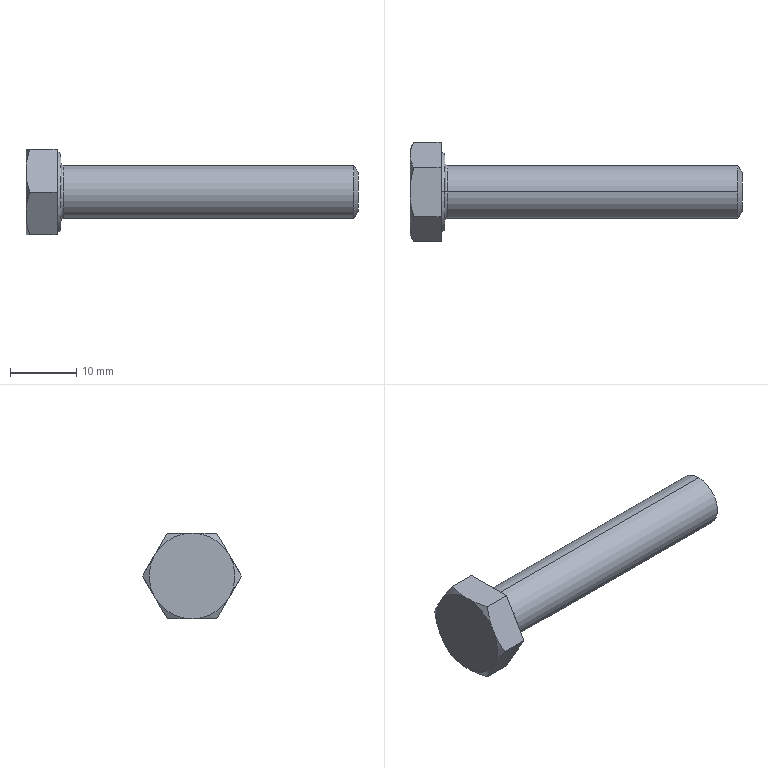Part | SolidWorks | features BaseBody 1 | 1 solid | 24 faces | box 50.3 x 15.011 x 13 mm | volume 3008 mm3 | cone 10 | plane 10 | spline 2 | cylinder 2 | commonest cylinder face diameters 8 x2
STEP:
#1=CARTESIAN_POINT('',(5.3,0.,4.4));
#2=VERTEX_POINT('',#1);
#3=CARTESIAN_POINT('',(5.3,0.,-4.4));
#4=VERTEX_POINT('',#3);
#5=CARTESIAN_POINT('',(5.3,0.,4.4));
#6=CARTESIAN_POINT('',(5.3,0.2797,4.4));
#7=CARTESIAN_POINT('',(5.3,0.6919,4.361));
#8=CARTESIAN_POINT('',(5.3,1.16,4.249));
#9=CARTESIAN_POINT('',(5.3,1.391,4.176));
#10=CARTESIAN_POINT('',(5.3,1.489,4.141));
#11=CARTESIAN_POINT('',(5.3,1.554,4.116));
#12=CARTESIAN_POINT('',(5.3,1.585,4.105));
#13=CARTESIAN_POINT('',(5.3,1.758,4.036));
#14=CARTESIAN_POINT('',(5.3,1.96,3.944));
#15=CARTESIAN_POINT('',(5.3,2.154,3.837));
#16=CARTESIAN_POINT('',(5.3,2.282,3.763));
#17=CARTESIAN_POINT('',(5.3,2.344,3.724));
#18=CARTESIAN_POINT('',(5.3,2.662,3.517));
#19=CARTESIAN_POINT('',(5.3,2.897,3.326));
#20=CARTESIAN_POINT('',(5.3,3.219,3.004));
#21=CARTESIAN_POINT('',(5.3,3.37,2.836));
#22=CARTESIAN_POINT('',(5.3,3.509,2.656));
#23=CARTESIAN_POINT('',(5.3,3.598,2.534));
#24=CARTESIAN_POINT('',(5.3,3.642,2.47));
#25=CARTESIAN_POINT('',(5.3,3.764,2.283));
#26=CARTESIAN_POINT('',(5.3,3.876,2.092));
#27=CARTESIAN_POINT('',(5.3,3.989,1.859));
#28=CARTESIAN_POINT('',(5.3,4.042,1.74));
#29=CARTESIAN_POINT('',(5.3,4.063,1.689));
#30=CARTESIAN_POINT('',(5.3,4.077,1.654));
#31=CARTESIAN_POINT('',(5.3,4.085,1.636));
#32=CARTESIAN_POINT('',(5.3,4.297,1.1));
#33=CARTESIAN_POINT('',(5.3,4.4,0.5592));
#34=CARTESIAN_POINT('',(5.3,4.4,-0.2796));
#35=CARTESIAN_POINT('',(5.3,4.361,-0.6917));
#36=CARTESIAN_POINT('',(5.3,4.249,-1.16));
#37=CARTESIAN_POINT('',(5.3,4.176,-1.391));
#38=CARTESIAN_POINT('',(5.3,4.141,-1.489));
#39=CARTESIAN_POINT('',(5.3,4.116,-1.554));
#40=CARTESIAN_POINT('',(5.3,4.105,-1.585));
#41=CARTESIAN_POINT('',(5.3,4.036,-1.758));
#42=CARTESIAN_POINT('',(5.3,3.944,-1.96));
#43=CARTESIAN_POINT('',(5.3,3.837,-2.154));
#44=CARTESIAN_POINT('',(5.3,3.763,-2.282));
#45=CARTESIAN_POINT('',(5.3,3.724,-2.344));
#46=CARTESIAN_POINT('',(5.3,3.517,-2.662));
#47=CARTESIAN_POINT('',(5.3,3.326,-2.897));
#48=CARTESIAN_POINT('',(5.3,3.004,-3.219));
#49=CARTESIAN_POINT('',(5.3,2.836,-3.37));
#50=CARTESIAN_POINT('',(5.3,2.656,-3.509));
#51=CARTESIAN_POINT('',(5.3,2.534,-3.598));
#52=CARTESIAN_POINT('',(5.3,2.47,-3.642));
#53=CARTESIAN_POINT('',(5.3,2.283,-3.764));
#54=CARTESIAN_POINT('',(5.3,2.092,-3.876));
#55=CARTESIAN_POINT('',(5.3,1.859,-3.989));
#56=CARTESIAN_POINT('',(5.3,1.74,-4.042));
#57=CARTESIAN_POINT('',(5.3,1.689,-4.063));
#58=CARTESIAN_POINT('',(5.3,1.654,-4.077));
#59=CARTESIAN_POINT('',(5.3,1.636,-4.085));
#60=CARTESIAN_POINT('',(5.3,1.1,-4.297));
#61=CARTESIAN_POINT('',(5.3,0.5597,-4.4));
#62=CARTESIAN_POINT('',(5.3,0.,-4.4));
#63=B_SPLINE_CURVE_WITH_KNOTS('',3,(#5,#6,#7,#8,#9,#10,#11,#12,#13,#14,#15,#16,#17,#18,#19,#20,#21,#22,#23,#24,#25,#26,#27,#28,#29,#30,#31,#32,#33,#34,#35,#36,#37,#38,#39,#40,#41,#42,#43,#44,#45,#46,#47,#48,#49,#50,#51,#52,#53,#54,#55,#56,#57,#58,#59,#60,#61,#62),.UNSPECIFIED.,.F.,.F.,(4,1,1,1,2,2,1,2,2,2,1,2,2,1,1,1,2,2,2,1,1,1,2,2,1,2,2,2,1,2,2,1,1,1,2,2,4),(0.,0.0625,0.09375,0.1094,0.1172,0.125,0.1562,0.1719,0.1875,0.25,0.2812,0.2969,0.3125,0.3437,0.3594,0.3672,0.3711,0.375,0.5,0.5625,0.5937,0.6094,0.6172,0.625,0.6562,0.6719,0.6875,0.75,0.7812,0.7969,0.8125,0.8437,0.8594,0.8672,0.8711,0.875,1.),.UNSPECIFIED.);
#64=EDGE_CURVE('',#2,#4,#63,.T.);
#65=ORIENTED_EDGE('',*,*,#64,.F.);
#66=CARTESIAN_POINT('',(5.7,0.,4.));
#67=VERTEX_POINT('',#66);
#68=CARTESIAN_POINT('',(5.7,0.,4.4));
#69=DIRECTION('',(0.,-1.,0.));
#70=DIRECTION('',(0.,0.,1.));
#71=AXIS2_PLACEMENT_3D('',#68,#69,#70);
#72=CIRCLE('',#71,0.4);
#73=EDGE_CURVE('',#2,#67,#72,.T.);
#74=ORIENTED_EDGE('',*,*,#73,.T.);
#75=CARTESIAN_POINT('',(5.7,0.,-4.));
#76=VERTEX_POINT('',#75);
#77=CARTESIAN_POINT('',(5.7,0.,0.));
#78=DIRECTION('',(1.,0.,0.));
#79=DIRECTION('',(0.,0.,1.));
#80=AXIS2_PLACEMENT_3D('',#77,#78,#79);
#81=CIRCLE('',#80,4.);
#82=EDGE_CURVE('',#76,#67,#81,.T.);
#83=ORIENTED_EDGE('',*,*,#82,.F.);
#84=CARTESIAN_POINT('',(5.7,0.,-4.4));
#85=DIRECTION('',(0.,1.,0.));
#86=DIRECTION('',(0.,0.,-1.));
#87=AXIS2_PLACEMENT_3D('',#84,#85,#86);
#88=CIRCLE('',#87,0.4);
#89=EDGE_CURVE('',#4,#76,#88,.T.);
#90=ORIENTED_EDGE('',*,*,#89,.F.);
#91=EDGE_LOOP('',(#65,#74,#83,#90));
#92=FACE_OUTER_BOUND('',#91,.T.);
#93=CARTESIAN_POINT('',(5.3,0.,-4.4));
#94=CARTESIAN_POINT('',(5.3,8.8,-4.4));
#95=CARTESIAN_POINT('',(5.3,8.8,4.4));
#96=CARTESIAN_POINT('',(5.3,0.,4.4));
#97=CARTESIAN_POINT('',(5.3,0.,-4.166));
#98=CARTESIAN_POINT('',(5.3,8.331,-4.166));
#99=CARTESIAN_POINT('',(5.3,8.331,4.166));
#100=CARTESIAN_POINT('',(5.3,0.,4.166));
#101=CARTESIAN_POINT('',(5.466,0.,-4.));
#102=CARTESIAN_POINT('',(5.466,8.,-4.));
#103=CARTESIAN_POINT('',(5.466,8.,4.));
#104=CARTESIAN_POINT('',(5.466,0.,4.));
#105=CARTESIAN_POINT('',(5.7,0.,-4.));
#106=CARTESIAN_POINT('',(5.7,8.,-4.));
#107=CARTESIAN_POINT('',(5.7,8.,4.));
#108=CARTESIAN_POINT('',(5.7,0.,4.));
#109=(BOUNDED_SURFACE()B_SPLINE_SURFACE(3,3,((#93,#94,#95,#96),(#97,#98,#99,#100),(#101,#102,#103,#104),(#105,#106,#107,#108)),.UNSPECIFIED.,.F.,.F.,.F.)B_SPLINE_SURFACE_WITH_KNOTS((4,4),(4,4),(0.,1.),(0.,1.),.UNSPECIFIED.)GEOMETRIC_REPRESENTATION_ITEM()RATIONAL_B_SPLINE_SURFACE(((1.,0.3333,0.3333,1.),(0.8047,0.2682,0.2682,0.8047),(0.8047,0.2682,0.2682,0.8047),(1.,0.3333,0.3333,1.)))REPRESENTATION_ITEM('')SURFACE());
#110=ADVANCED_FACE('',(#92),#109,.F.);
#111=CARTESIAN_POINT('',(49.675,0.,4.));
#112=VERTEX_POINT('',#111);
#113=CARTESIAN_POINT('',(49.675,0.,-4.));
#114=VERTEX_POINT('',#113);
#115=CARTESIAN_POINT('',(49.675,0.,0.));
#116=DIRECTION('',(-1.,0.,0.));
#117=DIRECTION('',(0.,0.,1.));
#118=AXIS2_PLACEMENT_3D('',#115,#116,#117);
#119=CIRCLE('',#118,4.);
#120=EDGE_CURVE('',#112,#114,#119,.T.);
#121=ORIENTED_EDGE('',*,*,#120,.T.);
#122=CARTESIAN_POINT('',(0.,0.,-4.));
#123=DIRECTION('',(-1.,0.,0.));
#124=VECTOR('',#123,1000.);
#125=LINE('',#122,#124);
#126=EDGE_CURVE('',#114,#76,#125,.T.);
#127=ORIENTED_EDGE('',*,*,#126,.T.);
#128=ORIENTED_EDGE('',*,*,#82,.T.);
#129=CARTESIAN_POINT('',(0.,0.,4.));
#130=DIRECTION('',(-1.,0.,0.));
#131=VECTOR('',#130,1000.);
#132=LINE('',#129,#131);
#133=EDGE_CURVE('',#112,#67,#132,.T.);
#134=ORIENTED_EDGE('',*,*,#133,.F.);
#135=EDGE_LOOP('',(#121,#127,#128,#134));
#136=FACE_OUTER_BOUND('',#135,.T.);
#137=CARTESIAN_POINT('',(0.,0.,0.));
#138=DIRECTION('',(-1.,0.,0.));
#139=DIRECTION('',(0.,0.,1.));
#140=AXIS2_PLACEMENT_3D('',#137,#138,#139);
#141=CYLINDRICAL_SURFACE('',#140,4.);
#142=ADVANCED_FACE('',(#136),#141,.T.);
#143=CARTESIAN_POINT('',(50.3,0.,2.917));
#144=VERTEX_POINT('',#143);
#145=CARTESIAN_POINT('',(50.3,0.,-2.917));
#146=VERTEX_POINT('',#145);
#147=CARTESIAN_POINT('',(50.3,0.,0.));
#148=DIRECTION('',(-1.,0.,0.));
#149=DIRECTION('',(0.,0.,1.));
#150=AXIS2_PLACEMENT_3D('',#147,#148,#149);
#151=CIRCLE('',#150,2.917);
#152=EDGE_CURVE('',#144,#146,#151,.T.);
#153=ORIENTED_EDGE('',*,*,#152,.T.);
#154=CARTESIAN_POINT('',(49.675,0.,-4.));
#155=DIRECTION('',(-0.5,0.,-0.866));
#156=VECTOR('',#155,1000.);
#157=LINE('',#154,#156);
#158=EDGE_CURVE('',#146,#114,#157,.T.);
#159=ORIENTED_EDGE('',*,*,#158,.T.);
#160=ORIENTED_EDGE('',*,*,#120,.F.);
#161=CARTESIAN_POINT('',(49.675,0.,4.));
#162=DIRECTION('',(-0.5,0.,0.866));
#163=VECTOR('',#162,1000.);
#164=LINE('',#161,#163);
#165=EDGE_CURVE('',#144,#112,#164,.T.);
#166=ORIENTED_EDGE('',*,*,#165,.F.);
#167=EDGE_LOOP('',(#153,#159,#160,#166));
#168=FACE_OUTER_BOUND('',#167,.T.);
#169=CARTESIAN_POINT('',(49.675,0.,0.));
#170=DIRECTION('',(-1.,0.,0.));
#171=DIRECTION('',(0.,0.,1.));
#172=AXIS2_PLACEMENT_3D('',#169,#170,#171);
#173=CONICAL_SURFACE('',#172,4.,1.047);
#174=ADVANCED_FACE('',(#168),#173,.T.);
#175=CARTESIAN_POINT('',(5.3,0.,-5.815));
#176=VERTEX_POINT('',#175);
#177=CARTESIAN_POINT('',(5.3,0.,5.815));
#178=VERTEX_POINT('',#177);
#179=CARTESIAN_POINT('',(5.3,0.,0.));
#180=DIRECTION('',(1.,0.,0.));
#181=DIRECTION('',(0.,0.,1.));
#182=AXIS2_PLACEMENT_3D('',#179,#180,#181);
#183=CIRCLE('',#182,5.815);
#184=EDGE_CURVE('',#176,#178,#183,.T.);
#185=ORIENTED_EDGE('',*,*,#184,.F.);
#186=CARTESIAN_POINT('',(4.7,0.,-6.161));
#187=VERTEX_POINT('',#186);
#188=CARTESIAN_POINT('',(4.7,0.,-6.161));
#189=DIRECTION('',(-0.866,0.,-0.5));
#190=VECTOR('',#189,1000.);
#191=LINE('',#188,#190);
#192=EDGE_CURVE('',#176,#187,#191,.T.);
#193=ORIENTED_EDGE('',*,*,#192,.T.);
#194=CARTESIAN_POINT('',(4.7,0.,6.161));
#195=VERTEX_POINT('',#194);
#196=CARTESIAN_POINT('',(4.7,0.,0.));
#197=DIRECTION('',(1.,0.,0.));
#198=DIRECTION('',(0.,0.,1.));
#199=AXIS2_PLACEMENT_3D('',#196,#197,#198);
#200=CIRCLE('',#199,6.161);
#201=EDGE_CURVE('',#187,#195,#200,.T.);
#202=ORIENTED_EDGE('',*,*,#201,.T.);
#203=CARTESIAN_POINT('',(4.7,0.,6.161));
#204=DIRECTION('',(-0.866,0.,0.5));
#205=VECTOR('',#204,1000.);
#206=LINE('',#203,#205);
#207=EDGE_CURVE('',#178,#195,#206,.T.);
#208=ORIENTED_EDGE('',*,*,#207,.F.);
#209=EDGE_LOOP('',(#185,#193,#202,#208));
#210=FACE_OUTER_BOUND('',#209,.T.);
#211=CARTESIAN_POINT('',(4.7,0.,0.));
#212=DIRECTION('',(-1.,0.,0.));
#213=DIRECTION('',(0.,0.,1.));
#214=AXIS2_PLACEMENT_3D('',#211,#212,#213);
#215=CONICAL_SURFACE('',#214,6.161,0.5236);
#216=ADVANCED_FACE('',(#210),#215,.T.);
#217=ORIENTED_EDGE('',*,*,#126,.F.);
#218=CARTESIAN_POINT('',(49.675,0.,0.));
#219=DIRECTION('',(-1.,0.,0.));
#220=DIRECTION('',(0.,0.,1.));
#221=AXIS2_PLACEMENT_3D('',#218,#219,#220);
#222=CIRCLE('',#221,4.);
#223=EDGE_CURVE('',#114,#112,#222,.T.);
#224=ORIENTED_EDGE('',*,*,#223,.T.);
#225=ORIENTED_EDGE('',*,*,#133,.T.);
#226=CARTESIAN_POINT('',(5.7,0.,0.));
#227=DIRECTION('',(1.,0.,0.));
#228=DIRECTION('',(0.,0.,1.));
#229=AXIS2_PLACEMENT_3D('',#226,#227,#228);
#230=CIRCLE('',#229,4.);
#231=EDGE_CURVE('',#67,#76,#230,.T.);
#232=ORIENTED_EDGE('',*,*,#231,.T.);
#233=EDGE_LOOP('',(#217,#224,#225,#232));
#234=FACE_OUTER_BOUND('',#233,.T.);
#235=CARTESIAN_POINT('',(0.,0.,0.));
#236=DIRECTION('',(-1.,0.,0.));
#237=DIRECTION('',(0.,0.,1.));
#238=AXIS2_PLACEMENT_3D('',#235,#236,#237);
#239=CYLINDRICAL_SURFACE('',#238,4.);
#240=ADVANCED_FACE('',(#234),#239,.T.);
#241=ORIENTED_EDGE('',*,*,#73,.F.);
#242=CARTESIAN_POINT('',(5.3,0.,-4.4));
#243=CARTESIAN_POINT('',(5.3,-0.2797,-4.4));
#244=CARTESIAN_POINT('',(5.3,-0.6919,-4.361));
#245=CARTESIAN_POINT('',(5.3,-1.16,-4.249));
#246=CARTESIAN_POINT('',(5.3,-1.391,-4.176));
#247=CARTESIAN_POINT('',(5.3,-1.489,-4.141));
#248=CARTESIAN_POINT('',(5.3,-1.554,-4.116));
#249=CARTESIAN_POINT('',(5.3,-1.585,-4.105));
#250=CARTESIAN_POINT('',(5.3,-1.758,-4.036));
#251=CARTESIAN_POINT('',(5.3,-1.96,-3.944));
#252=CARTESIAN_POINT('',(5.3,-2.154,-3.837));
#253=CARTESIAN_POINT('',(5.3,-2.282,-3.763));
#254=CARTESIAN_POINT('',(5.3,-2.344,-3.724));
#255=CARTESIAN_POINT('',(5.3,-2.662,-3.517));
#256=CARTESIAN_POINT('',(5.3,-2.897,-3.326));
#257=CARTESIAN_POINT('',(5.3,-3.219,-3.004));
#258=CARTESIAN_POINT('',(5.3,-3.37,-2.836));
#259=CARTESIAN_POINT('',(5.3,-3.509,-2.656));
#260=CARTESIAN_POINT('',(5.3,-3.598,-2.534));
#261=CARTESIAN_POINT('',(5.3,-3.642,-2.47));
#262=CARTESIAN_POINT('',(5.3,-3.764,-2.283));
#263=CARTESIAN_POINT('',(5.3,-3.876,-2.092));
#264=CARTESIAN_POINT('',(5.3,-3.989,-1.859));
#265=CARTESIAN_POINT('',(5.3,-4.042,-1.74));
#266=CARTESIAN_POINT('',(5.3,-4.063,-1.689));
#267=CARTESIAN_POINT('',(5.3,-4.077,-1.654));
#268=CARTESIAN_POINT('',(5.3,-4.085,-1.636));
#269=CARTESIAN_POINT('',(5.3,-4.297,-1.1));
#270=CARTESIAN_POINT('',(5.3,-4.4,-0.5592));
#271=CARTESIAN_POINT('',(5.3,-4.4,0.2796));
#272=CARTESIAN_POINT('',(5.3,-4.361,0.6917));
#273=CARTESIAN_POINT('',(5.3,-4.249,1.16));
#274=CARTESIAN_POINT('',(5.3,-4.176,1.391));
#275=CARTESIAN_POINT('',(5.3,-4.141,1.489));
#276=CARTESIAN_POINT('',(5.3,-4.116,1.554));
#277=CARTESIAN_POINT('',(5.3,-4.105,1.585));
#278=CARTESIAN_POINT('',(5.3,-4.036,1.758));
#279=CARTESIAN_POINT('',(5.3,-3.944,1.96));
#280=CARTESIAN_POINT('',(5.3,-3.837,2.154));
#281=CARTESIAN_POINT('',(5.3,-3.763,2.282));
#282=CARTESIAN_POINT('',(5.3,-3.724,2.344));
#283=CARTESIAN_POINT('',(5.3,-3.517,2.662));
#284=CARTESIAN_POINT('',(5.3,-3.326,2.897));
#285=CARTESIAN_POINT('',(5.3,-3.004,3.219));
#286=CARTESIAN_POINT('',(5.3,-2.836,3.37));
#287=CARTESIAN_POINT('',(5.3,-2.656,3.509));
#288=CARTESIAN_POINT('',(5.3,-2.534,3.598));
#289=CARTESIAN_POINT('',(5.3,-2.47,3.642));
#290=CARTESIAN_POINT('',(5.3,-2.283,3.764));
#291=CARTESIAN_POINT('',(5.3,-2.092,3.876));
#292=CARTESIAN_POINT('',(5.3,-1.859,3.989));
#293=CARTESIAN_POINT('',(5.3,-1.74,4.042));
#294=CARTESIAN_POINT('',(5.3,-1.689,4.063));
#295=CARTESIAN_POINT('',(5.3,-1.654,4.077));
#296=CARTESIAN_POINT('',(5.3,-1.636,4.085));
#297=CARTESIAN_POINT('',(5.3,-1.1,4.297));
#298=CARTESIAN_POINT('',(5.3,-0.5597,4.4));
#299=CARTESIAN_POINT('',(5.3,0.,4.4));
#300=B_SPLINE_CURVE_WITH_KNOTS('',3,(#242,#243,#244,#245,#246,#247,#248,#249,#250,#251,#252,#253,#254,#255,#256,#257,#258,#259,#260,#261,#262,#263,#264,#265,#266,#267,#268,#269,#270,#271,#272,#273,#274,#275,#276,#277,#278,#279,#280,#281,#282,#283,#284,#285,#286,#287,#288,#289,#290,#291,#292,#293,#294,#295,#296,#297,#298,#299),.UNSPECIFIED.,.F.,.F.,(4,1,1,1,2,2,1,2,2,2,1,2,2,1,1,1,2,2,2,1,1,1,2,2,1,2,2,2,1,2,2,1,1,1,2,2,4),(0.,0.0625,0.09375,0.1094,0.1172,0.125,0.1562,0.1719,0.1875,0.25,0.2812,0.2969,0.3125,0.3437,0.3594,0.3672,0.3711,0.375,0.5,0.5625,0.5937,0.6094,0.6172,0.625,0.6562,0.6719,0.6875,0.75,0.7812,0.7969,0.8125,0.8437,0.8594,0.8672,0.8711,0.875,1.),.UNSPECIFIED.);
#301=EDGE_CURVE('',#4,#2,#300,.T.);
#302=ORIENTED_EDGE('',*,*,#301,.F.);
#303=ORIENTED_EDGE('',*,*,#89,.T.);
#304=ORIENTED_EDGE('',*,*,#231,.F.);
#305=EDGE_LOOP('',(#241,#302,#303,#304));
#306=FACE_OUTER_BOUND('',#305,.T.);
#307=CARTESIAN_POINT('',(5.3,0.,4.4));
#308=CARTESIAN_POINT('',(5.3,-8.8,4.4));
#309=CARTESIAN_POINT('',(5.3,-8.8,-4.4));
#310=CARTESIAN_POINT('',(5.3,0.,-4.4));
#311=CARTESIAN_POINT('',(5.3,0.,4.166));
#312=CARTESIAN_POINT('',(5.3,-8.331,4.166));
#313=CARTESIAN_POINT('',(5.3,-8.331,-4.166));
#314=CARTESIAN_POINT('',(5.3,0.,-4.166));
#315=CARTESIAN_POINT('',(5.466,0.,4.));
#316=CARTESIAN_POINT('',(5.466,-8.,4.));
#317=CARTESIAN_POINT('',(5.466,-8.,-4.));
#318=CARTESIAN_POINT('',(5.466,0.,-4.));
#319=CARTESIAN_POINT('',(5.7,0.,4.));
#320=CARTESIAN_POINT('',(5.7,-8.,4.));
#321=CARTESIAN_POINT('',(5.7,-8.,-4.));
#322=CARTESIAN_POINT('',(5.7,0.,-4.));
#323=(BOUNDED_SURFACE()B_SPLINE_SURFACE(3,3,((#307,#308,#309,#310),(#311,#312,#313,#314),(#315,#316,#317,#318),(#319,#320,#321,#322)),.UNSPECIFIED.,.F.,.F.,.T.)B_SPLINE_SURFACE_WITH_KNOTS((4,4),(4,4),(0.,1.),(0.,1.),.UNSPECIFIED.)GEOMETRIC_REPRESENTATION_ITEM()RATIONAL_B_SPLINE_SURFACE(((1.,0.3333,0.3333,1.),(0.8047,0.2682,0.2682,0.8047),(0.8047,0.2682,0.2682,0.8047),(1.,0.3333,0.3333,1.)))REPRESENTATION_ITEM('')SURFACE());
#324=ADVANCED_FACE('',(#306),#323,.F.);
#325=ORIENTED_EDGE('',*,*,#158,.F.);
#326=CARTESIAN_POINT('',(50.3,0.,0.));
#327=DIRECTION('',(-1.,0.,0.));
#328=DIRECTION('',(0.,0.,1.));
#329=AXIS2_PLACEMENT_3D('',#326,#327,#328);
#330=CIRCLE('',#329,2.917);
#331=EDGE_CURVE('',#146,#144,#330,.T.);
#332=ORIENTED_EDGE('',*,*,#331,.T.);
#333=ORIENTED_EDGE('',*,*,#165,.T.);
#334=ORIENTED_EDGE('',*,*,#223,.F.);
#335=EDGE_LOOP('',(#325,#332,#333,#334));
#336=FACE_OUTER_BOUND('',#335,.T.);
#337=CARTESIAN_POINT('',(49.675,0.,0.));
#338=DIRECTION('',(-1.,0.,0.));
#339=DIRECTION('',(0.,0.,1.));
#340=AXIS2_PLACEMENT_3D('',#337,#338,#339);
#341=CONICAL_SURFACE('',#340,4.,1.047);
#342=ADVANCED_FACE('',(#336),#341,.T.);
#343=CARTESIAN_POINT('',(5.3,0.,0.));
#344=DIRECTION('',(1.,0.,0.));
#345=DIRECTION('',(0.,0.,1.));
#346=AXIS2_PLACEMENT_3D('',#343,#344,#345);
#347=CIRCLE('',#346,5.815);
#348=EDGE_CURVE('',#178,#176,#347,.T.);
#349=ORIENTED_EDGE('',*,*,#348,.T.);
#350=ORIENTED_EDGE('',*,*,#184,.T.);
#351=EDGE_LOOP('',(#349,#350));
#352=FACE_OUTER_BOUND('',#351,.T.);
#353=ORIENTED_EDGE('',*,*,#301,.T.);
#354=ORIENTED_EDGE('',*,*,#64,.T.);
#355=EDGE_LOOP('',(#353,#354));
#356=FACE_BOUND('',#355,.T.);
#357=CARTESIAN_POINT('',(5.3,0.,-13.));
#358=DIRECTION('',(1.,0.,0.));
#359=DIRECTION('',(0.,0.,-1.));
#360=AXIS2_PLACEMENT_3D('',#357,#358,#359);
#361=PLANE('',#360);
#362=ADVANCED_FACE('',(#352,#356),#361,.T.);
#363=ORIENTED_EDGE('',*,*,#152,.F.);
#364=ORIENTED_EDGE('',*,*,#331,.F.);
#365=EDGE_LOOP('',(#363,#364));
#366=FACE_OUTER_BOUND('',#365,.T.);
#367=CARTESIAN_POINT('',(50.3,0.,0.));
#368=DIRECTION('',(-1.,0.,0.));
#369=DIRECTION('',(0.,0.,1.));
#370=AXIS2_PLACEMENT_3D('',#367,#368,#369);
#371=PLANE('',#370);
#372=ADVANCED_FACE('',(#366),#371,.F.);
#373=ORIENTED_EDGE('',*,*,#192,.F.);
#374=ORIENTED_EDGE('',*,*,#348,.F.);
#375=ORIENTED_EDGE('',*,*,#207,.T.);
#376=CARTESIAN_POINT('',(4.7,0.,0.));
#377=DIRECTION('',(1.,0.,0.));
#378=DIRECTION('',(0.,0.,1.));
#379=AXIS2_PLACEMENT_3D('',#376,#377,#378);
#380=CIRCLE('',#379,6.161);
#381=EDGE_CURVE('',#195,#187,#380,.T.);
#382=ORIENTED_EDGE('',*,*,#381,.T.);
#383=EDGE_LOOP('',(#373,#374,#375,#382));
#384=FACE_OUTER_BOUND('',#383,.T.);
#385=CARTESIAN_POINT('',(4.7,0.,0.));
#386=DIRECTION('',(-1.,0.,0.));
#387=DIRECTION('',(0.,0.,1.));
#388=AXIS2_PLACEMENT_3D('',#385,#386,#387);
#389=CONICAL_SURFACE('',#388,6.161,0.5236);
#390=ADVANCED_FACE('',(#384),#389,.T.);
#391=CARTESIAN_POINT('',(4.7,-7.506,0.));
#392=VERTEX_POINT('',#391);
#393=CARTESIAN_POINT('',(4.7,-3.753,-6.5));
#394=VERTEX_POINT('',#393);
#395=CARTESIAN_POINT('',(4.7,-7.506,0.));
#396=DIRECTION('',(0.,0.5,-0.866));
#397=VECTOR('',#396,1000.);
#398=LINE('',#395,#397);
#399=EDGE_CURVE('',#392,#394,#398,.T.);
#400=ORIENTED_EDGE('',*,*,#399,.T.);
#401=CARTESIAN_POINT('',(4.7,3.753,-6.5));
#402=VERTEX_POINT('',#401);
#403=CARTESIAN_POINT('',(4.7,6.161,-6.5));
#404=DIRECTION('',(0.,1.,0.));
#405=VECTOR('',#404,1000.);
#406=LINE('',#403,#405);
#407=EDGE_CURVE('',#394,#402,#406,.T.);
#408=ORIENTED_EDGE('',*,*,#407,.T.);
#409=CARTESIAN_POINT('',(4.7,7.506,0.));
#410=VERTEX_POINT('',#409);
#411=CARTESIAN_POINT('',(4.7,3.753,-6.5));
#412=DIRECTION('',(0.,0.5,0.866));
#413=VECTOR('',#412,1000.);
#414=LINE('',#411,#413);
#415=EDGE_CURVE('',#402,#410,#414,.T.);
#416=ORIENTED_EDGE('',*,*,#415,.T.);
#417=CARTESIAN_POINT('',(4.7,3.753,6.5));
#418=VERTEX_POINT('',#417);
#419=CARTESIAN_POINT('',(4.7,7.506,0.));
#420=DIRECTION('',(0.,-0.5,0.866));
#421=VECTOR('',#420,1000.);
#422=LINE('',#419,#421);
#423=EDGE_CURVE('',#410,#418,#422,.T.);
#424=ORIENTED_EDGE('',*,*,#423,.T.);
#425=CARTESIAN_POINT('',(4.7,-3.753,6.5));
#426=VERTEX_POINT('',#425);
#427=CARTESIAN_POINT('',(4.7,6.161,6.5));
#428=DIRECTION('',(0.,-1.,0.));
#429=VECTOR('',#428,1000.);
#430=LINE('',#427,#429);
#431=EDGE_CURVE('',#418,#426,#430,.T.);
#432=ORIENTED_EDGE('',*,*,#431,.T.);
#433=CARTESIAN_POINT('',(4.7,-3.753,6.5));
#434=DIRECTION('',(0.,-0.5,-0.866));
#435=VECTOR('',#434,1000.);
#436=LINE('',#433,#435);
#437=EDGE_CURVE('',#426,#392,#436,.T.);
#438=ORIENTED_EDGE('',*,*,#437,.T.);
#439=EDGE_LOOP('',(#400,#408,#416,#424,#432,#438));
#440=FACE_OUTER_BOUND('',#439,.T.);
#441=ORIENTED_EDGE('',*,*,#381,.F.);
#442=ORIENTED_EDGE('',*,*,#201,.F.);
#443=EDGE_LOOP('',(#441,#442));
#444=FACE_BOUND('',#443,.T.);
#445=CARTESIAN_POINT('',(4.7,6.161,0.));
#446=DIRECTION('',(1.,0.,0.));
#447=DIRECTION('',(0.,0.,-1.));
#448=AXIS2_PLACEMENT_3D('',#445,#446,#447);
#449=PLANE('',#448);
#450=ADVANCED_FACE('',(#440,#444),#449,.T.);
#451=CARTESIAN_POINT('',(0.5806,-3.753,-6.5));
#452=VERTEX_POINT('',#451);
#453=CARTESIAN_POINT('',(5.3,-3.753,-6.5));
#454=DIRECTION('',(1.,0.,0.));
#455=VECTOR('',#454,1000.);
#456=LINE('',#453,#455);
#457=EDGE_CURVE('',#452,#394,#456,.T.);
#458=ORIENTED_EDGE('',*,*,#457,.F.);
#459=CARTESIAN_POINT('',(0.,0.,-6.5));
#460=VERTEX_POINT('',#459);
#461=CARTESIAN_POINT('',(0.,0.,-6.5));
#462=CARTESIAN_POINT('',(0.,-1.281,-6.5));
#463=CARTESIAN_POINT('',(0.2266,-2.527,-6.5));
#464=CARTESIAN_POINT('',(0.5806,-3.753,-6.5));
#465=B_SPLINE_CURVE_WITH_KNOTS('',3,(#461,#462,#463,#464),.UNSPECIFIED.,.F.,.F.,(4,4),(0.,0.003797),.UNSPECIFIED.);
#466=EDGE_CURVE('',#460,#452,#465,.T.);
#467=ORIENTED_EDGE('',*,*,#466,.F.);
#468=CARTESIAN_POINT('',(0.5806,3.753,-6.5));
#469=VERTEX_POINT('',#468);
#470=CARTESIAN_POINT('',(0.5806,3.753,-6.5));
#471=CARTESIAN_POINT('',(0.2266,2.527,-6.5));
#472=CARTESIAN_POINT('',(0.,1.281,-6.5));
#473=CARTESIAN_POINT('',(0.,0.,-6.5));
#474=B_SPLINE_CURVE_WITH_KNOTS('',3,(#470,#471,#472,#473),.UNSPECIFIED.,.F.,.F.,(4,4),(0.,0.003797),.UNSPECIFIED.);
#475=EDGE_CURVE('',#469,#460,#474,.T.);
#476=ORIENTED_EDGE('',*,*,#475,.F.);
#477=CARTESIAN_POINT('',(5.3,3.753,-6.5));
#478=DIRECTION('',(-1.,0.,0.));
#479=VECTOR('',#478,1000.);
#480=LINE('',#477,#479);
#481=EDGE_CURVE('',#402,#469,#480,.T.);
#482=ORIENTED_EDGE('',*,*,#481,.F.);
#483=ORIENTED_EDGE('',*,*,#407,.F.);
#484=EDGE_LOOP('',(#458,#467,#476,#482,#483));
#485=FACE_OUTER_BOUND('',#484,.T.);
#486=CARTESIAN_POINT('',(5.3,3.753,-6.5));
#487=DIRECTION('',(0.,0.,1.));
#488=DIRECTION('',(1.,0.,0.));
#489=AXIS2_PLACEMENT_3D('',#486,#487,#488);
#490=PLANE('',#489);
#491=ADVANCED_FACE('',(#485),#490,.F.);
#492=CARTESIAN_POINT('',(0.5806,-7.506,0.));
#493=VERTEX_POINT('',#492);
#494=CARTESIAN_POINT('',(5.3,-7.506,0.));
#495=DIRECTION('',(1.,0.,0.));
#496=VECTOR('',#495,1000.);
#497=LINE('',#494,#496);
#498=EDGE_CURVE('',#493,#392,#497,.T.);
#499=ORIENTED_EDGE('',*,*,#498,.F.);
#500=CARTESIAN_POINT('',(0.,-5.629,-3.25));
#501=VERTEX_POINT('',#500);
#502=CARTESIAN_POINT('',(0.,-5.629,-3.25));
#503=CARTESIAN_POINT('',(0.,-6.27,-2.141));
#504=CARTESIAN_POINT('',(0.2266,-6.892,-1.062));
#505=CARTESIAN_POINT('',(0.5806,-7.506,0.));
#506=B_SPLINE_CURVE_WITH_KNOTS('',3,(#502,#503,#504,#505),.UNSPECIFIED.,.F.,.F.,(4,4),(0.,0.003797),.UNSPECIFIED.);
#507=EDGE_CURVE('',#501,#493,#506,.T.);
#508=ORIENTED_EDGE('',*,*,#507,.F.);
#509=CARTESIAN_POINT('',(0.5806,-3.753,-6.5));
#510=CARTESIAN_POINT('',(0.2266,-4.366,-5.438));
#511=CARTESIAN_POINT('',(0.,-4.989,-4.359));
#512=CARTESIAN_POINT('',(0.,-5.629,-3.25));
#513=B_SPLINE_CURVE_WITH_KNOTS('',3,(#509,#510,#511,#512),.UNSPECIFIED.,.F.,.F.,(4,4),(0.,0.003797),.UNSPECIFIED.);
#514=EDGE_CURVE('',#452,#501,#513,.T.);
#515=ORIENTED_EDGE('',*,*,#514,.F.);
#516=ORIENTED_EDGE('',*,*,#457,.T.);
#517=ORIENTED_EDGE('',*,*,#399,.F.);
#518=EDGE_LOOP('',(#499,#508,#515,#516,#517));
#519=FACE_OUTER_BOUND('',#518,.T.);
#520=CARTESIAN_POINT('',(5.3,-3.753,-6.5));
#521=DIRECTION('',(0.,0.866,0.5));
#522=DIRECTION('',(0.,-0.5,0.866));
#523=AXIS2_PLACEMENT_3D('',#520,#521,#522);
#524=PLANE('',#523);
#525=ADVANCED_FACE('',(#519),#524,.F.);
#526=CARTESIAN_POINT('',(0.5806,-3.753,6.5));
#527=VERTEX_POINT('',#526);
#528=CARTESIAN_POINT('',(5.3,-3.753,6.5));
#529=DIRECTION('',(1.,0.,0.));
#530=VECTOR('',#529,1000.);
#531=LINE('',#528,#530);
#532=EDGE_CURVE('',#527,#426,#531,.T.);
#533=ORIENTED_EDGE('',*,*,#532,.F.);
#534=CARTESIAN_POINT('',(0.,-5.629,3.25));
#535=VERTEX_POINT('',#534);
#536=CARTESIAN_POINT('',(0.,-5.629,3.25));
#537=CARTESIAN_POINT('',(0.,-4.989,4.359));
#538=CARTESIAN_POINT('',(0.2266,-4.366,5.438));
#539=CARTESIAN_POINT('',(0.5806,-3.753,6.5));
#540=B_SPLINE_CURVE_WITH_KNOTS('',3,(#536,#537,#538,#539),.UNSPECIFIED.,.F.,.F.,(4,4),(0.,0.003797),.UNSPECIFIED.);
#541=EDGE_CURVE('',#535,#527,#540,.T.);
#542=ORIENTED_EDGE('',*,*,#541,.F.);
#543=CARTESIAN_POINT('',(0.5806,-7.506,0.));
#544=CARTESIAN_POINT('',(0.2266,-6.892,1.062));
#545=CARTESIAN_POINT('',(0.,-6.27,2.141));
#546=CARTESIAN_POINT('',(0.,-5.629,3.25));
#547=B_SPLINE_CURVE_WITH_KNOTS('',3,(#543,#544,#545,#546),.UNSPECIFIED.,.F.,.F.,(4,4),(0.,0.003797),.UNSPECIFIED.);
#548=EDGE_CURVE('',#493,#535,#547,.T.);
#549=ORIENTED_EDGE('',*,*,#548,.F.);
#550=ORIENTED_EDGE('',*,*,#498,.T.);
#551=ORIENTED_EDGE('',*,*,#437,.F.);
#552=EDGE_LOOP('',(#533,#542,#549,#550,#551));
#553=FACE_OUTER_BOUND('',#552,.T.);
#554=CARTESIAN_POINT('',(5.3,-7.506,0.));
#555=DIRECTION('',(0.,0.866,-0.5));
#556=DIRECTION('',(0.,0.5,0.866));
#557=AXIS2_PLACEMENT_3D('',#554,#555,#556);
#558=PLANE('',#557);
#559=ADVANCED_FACE('',(#553),#558,.F.);
#560=CARTESIAN_POINT('',(0.5806,3.753,6.5));
#561=VERTEX_POINT('',#560);
#562=CARTESIAN_POINT('',(5.3,3.753,6.5));
#563=DIRECTION('',(1.,0.,0.));
#564=VECTOR('',#563,1000.);
#565=LINE('',#562,#564);
#566=EDGE_CURVE('',#561,#418,#565,.T.);
#567=ORIENTED_EDGE('',*,*,#566,.F.);
#568=CARTESIAN_POINT('',(0.,0.,6.5));
#569=VERTEX_POINT('',#568);
#570=CARTESIAN_POINT('',(0.,0.,6.5));
#571=CARTESIAN_POINT('',(0.,1.281,6.5));
#572=CARTESIAN_POINT('',(0.2266,2.527,6.5));
#573=CARTESIAN_POINT('',(0.5806,3.753,6.5));
#574=B_SPLINE_CURVE_WITH_KNOTS('',3,(#570,#571,#572,#573),.UNSPECIFIED.,.F.,.F.,(4,4),(0.,0.003797),.UNSPECIFIED.);
#575=EDGE_CURVE('',#569,#561,#574,.T.);
#576=ORIENTED_EDGE('',*,*,#575,.F.);
#577=CARTESIAN_POINT('',(0.5806,-3.753,6.5));
#578=CARTESIAN_POINT('',(0.2266,-2.527,6.5));
#579=CARTESIAN_POINT('',(0.,-1.281,6.5));
#580=CARTESIAN_POINT('',(0.,0.,6.5));
#581=B_SPLINE_CURVE_WITH_KNOTS('',3,(#577,#578,#579,#580),.UNSPECIFIED.,.F.,.F.,(4,4),(0.,0.003797),.UNSPECIFIED.);
#582=EDGE_CURVE('',#527,#569,#581,.T.);
#583=ORIENTED_EDGE('',*,*,#582,.F.);
#584=ORIENTED_EDGE('',*,*,#532,.T.);
#585=ORIENTED_EDGE('',*,*,#431,.F.);
#586=EDGE_LOOP('',(#567,#576,#583,#584,#585));
#587=FACE_OUTER_BOUND('',#586,.T.);
#588=CARTESIAN_POINT('',(5.3,3.753,6.5));
#589=DIRECTION('',(0.,0.,-1.));
#590=DIRECTION('',(-1.,0.,0.));
#591=AXIS2_PLACEMENT_3D('',#588,#589,#590);
#592=PLANE('',#591);
#593=ADVANCED_FACE('',(#587),#592,.F.);
#594=CARTESIAN_POINT('',(0.5806,7.506,0.));
#595=VERTEX_POINT('',#594);
#596=CARTESIAN_POINT('',(5.3,7.506,0.));
#597=DIRECTION('',(1.,0.,0.));
#598=VECTOR('',#597,1000.);
#599=LINE('',#596,#598);
#600=EDGE_CURVE('',#595,#410,#599,.T.);
#601=ORIENTED_EDGE('',*,*,#600,.F.);
#602=CARTESIAN_POINT('',(0.,5.629,3.25));
#603=VERTEX_POINT('',#602);
#604=CARTESIAN_POINT('',(0.,5.629,3.25));
#605=CARTESIAN_POINT('',(0.,6.27,2.141));
#606=CARTESIAN_POINT('',(0.2266,6.892,1.062));
#607=CARTESIAN_POINT('',(0.5806,7.506,0.));
#608=B_SPLINE_CURVE_WITH_KNOTS('',3,(#604,#605,#606,#607),.UNSPECIFIED.,.F.,.F.,(4,4),(0.,0.003797),.UNSPECIFIED.);
#609=EDGE_CURVE('',#603,#595,#608,.T.);
#610=ORIENTED_EDGE('',*,*,#609,.F.);
#611=CARTESIAN_POINT('',(0.5806,3.753,6.5));
#612=CARTESIAN_POINT('',(0.2266,4.366,5.438));
#613=CARTESIAN_POINT('',(0.,4.989,4.359));
#614=CARTESIAN_POINT('',(0.,5.629,3.25));
#615=B_SPLINE_CURVE_WITH_KNOTS('',3,(#611,#612,#613,#614),.UNSPECIFIED.,.F.,.F.,(4,4),(0.,0.003797),.UNSPECIFIED.);
#616=EDGE_CURVE('',#561,#603,#615,.T.);
#617=ORIENTED_EDGE('',*,*,#616,.F.);
#618=ORIENTED_EDGE('',*,*,#566,.T.);
#619=ORIENTED_EDGE('',*,*,#423,.F.);
#620=EDGE_LOOP('',(#601,#610,#617,#618,#619));
#621=FACE_OUTER_BOUND('',#620,.T.);
#622=CARTESIAN_POINT('',(5.3,7.506,0.));
#623=DIRECTION('',(0.,-0.866,-0.5));
#624=DIRECTION('',(0.,0.5,-0.866));
#625=AXIS2_PLACEMENT_3D('',#622,#623,#624);
#626=PLANE('',#625);
#627=ADVANCED_FACE('',(#621),#626,.F.);
#628=ORIENTED_EDGE('',*,*,#481,.T.);
#629=CARTESIAN_POINT('',(0.,5.629,-3.25));
#630=VERTEX_POINT('',#629);
#631=CARTESIAN_POINT('',(0.,5.629,-3.25));
#632=CARTESIAN_POINT('',(0.,4.989,-4.359));
#633=CARTESIAN_POINT('',(0.2266,4.366,-5.438));
#634=CARTESIAN_POINT('',(0.5806,3.753,-6.5));
#635=B_SPLINE_CURVE_WITH_KNOTS('',3,(#631,#632,#633,#634),.UNSPECIFIED.,.F.,.F.,(4,4),(0.,0.003797),.UNSPECIFIED.);
#636=EDGE_CURVE('',#630,#469,#635,.T.);
#637=ORIENTED_EDGE('',*,*,#636,.F.);
#638=CARTESIAN_POINT('',(0.5806,7.506,0.));
#639=CARTESIAN_POINT('',(0.2266,6.892,-1.062));
#640=CARTESIAN_POINT('',(0.,6.27,-2.141));
#641=CARTESIAN_POINT('',(0.,5.629,-3.25));
#642=B_SPLINE_CURVE_WITH_KNOTS('',3,(#638,#639,#640,#641),.UNSPECIFIED.,.F.,.F.,(4,4),(0.,0.003797),.UNSPECIFIED.);
#643=EDGE_CURVE('',#595,#630,#642,.T.);
#644=ORIENTED_EDGE('',*,*,#643,.F.);
#645=ORIENTED_EDGE('',*,*,#600,.T.);
#646=ORIENTED_EDGE('',*,*,#415,.F.);
#647=EDGE_LOOP('',(#628,#637,#644,#645,#646));
#648=FACE_OUTER_BOUND('',#647,.T.);
#649=CARTESIAN_POINT('',(5.3,3.753,-6.5));
#650=DIRECTION('',(0.,-0.866,0.5));
#651=DIRECTION('',(0.,-0.5,-0.866));
#652=AXIS2_PLACEMENT_3D('',#649,#650,#651);
#653=PLANE('',#652);
#654=ADVANCED_FACE('',(#648),#653,.F.);
#655=CARTESIAN_POINT('',(0.,0.,0.));
#656=DIRECTION('',(1.,0.,0.));
#657=DIRECTION('',(0.,0.,-1.));
#658=AXIS2_PLACEMENT_3D('',#655,#656,#657);
#659=CIRCLE('',#658,6.5);
#660=EDGE_CURVE('',#501,#460,#659,.T.);
#661=ORIENTED_EDGE('',*,*,#660,.T.);
#662=ORIENTED_EDGE('',*,*,#466,.T.);
#663=ORIENTED_EDGE('',*,*,#514,.T.);
#664=EDGE_LOOP('',(#661,#662,#663));
#665=FACE_OUTER_BOUND('',#664,.T.);
#666=CARTESIAN_POINT('',(0.584,0.,0.));
#667=DIRECTION('',(1.,0.,0.));
#668=DIRECTION('',(0.,0.,-1.));
#669=AXIS2_PLACEMENT_3D('',#666,#667,#668);
#670=CONICAL_SURFACE('',#669,7.512,1.047);
#671=ADVANCED_FACE('',(#665),#670,.T.);
#672=ORIENTED_EDGE('',*,*,#475,.T.);
#673=CARTESIAN_POINT('',(0.,0.,0.));
#674=DIRECTION('',(1.,0.,0.));
#675=DIRECTION('',(0.,0.,-1.));
#676=AXIS2_PLACEMENT_3D('',#673,#674,#675);
#677=CIRCLE('',#676,6.5);
#678=EDGE_CURVE('',#460,#630,#677,.T.);
#679=ORIENTED_EDGE('',*,*,#678,.T.);
#680=ORIENTED_EDGE('',*,*,#636,.T.);
#681=EDGE_LOOP('',(#672,#679,#680));
#682=FACE_OUTER_BOUND('',#681,.T.);
#683=CARTESIAN_POINT('',(0.584,0.,0.));
#684=DIRECTION('',(1.,0.,0.));
#685=DIRECTION('',(0.,0.,-1.));
#686=AXIS2_PLACEMENT_3D('',#683,#684,#685);
#687=CONICAL_SURFACE('',#686,7.512,1.047);
#688=ADVANCED_FACE('',(#682),#687,.T.);
#689=CARTESIAN_POINT('',(0.,0.,0.));
#690=DIRECTION('',(1.,0.,0.));
#691=DIRECTION('',(0.,0.,-1.));
#692=AXIS2_PLACEMENT_3D('',#689,#690,#691);
#693=CIRCLE('',#692,6.5);
#694=EDGE_CURVE('',#535,#501,#693,.T.);
#695=ORIENTED_EDGE('',*,*,#694,.T.);
#696=ORIENTED_EDGE('',*,*,#507,.T.);
#697=ORIENTED_EDGE('',*,*,#548,.T.);
#698=EDGE_LOOP('',(#695,#696,#697));
#699=FACE_OUTER_BOUND('',#698,.T.);
#700=CARTESIAN_POINT('',(0.584,0.,0.));
#701=DIRECTION('',(1.,0.,0.));
#702=DIRECTION('',(0.,0.,-1.));
#703=AXIS2_PLACEMENT_3D('',#700,#701,#702);
#704=CONICAL_SURFACE('',#703,7.512,1.047);
#705=ADVANCED_FACE('',(#699),#704,.T.);
#706=CARTESIAN_POINT('',(0.,0.,0.));
#707=DIRECTION('',(1.,0.,0.));
#708=DIRECTION('',(0.,0.,-1.));
#709=AXIS2_PLACEMENT_3D('',#706,#707,#708);
#710=CIRCLE('',#709,6.5);
#711=EDGE_CURVE('',#569,#535,#710,.T.);
#712=ORIENTED_EDGE('',*,*,#711,.T.);
#713=ORIENTED_EDGE('',*,*,#541,.T.);
#714=ORIENTED_EDGE('',*,*,#582,.T.);
#715=EDGE_LOOP('',(#712,#713,#714));
#716=FACE_OUTER_BOUND('',#715,.T.);
#717=CARTESIAN_POINT('',(0.584,0.,0.));
#718=DIRECTION('',(1.,0.,0.));
#719=DIRECTION('',(0.,0.,-1.));
#720=AXIS2_PLACEMENT_3D('',#717,#718,#719);
#721=CONICAL_SURFACE('',#720,7.512,1.047);
#722=ADVANCED_FACE('',(#716),#721,.T.);
#723=ORIENTED_EDGE('',*,*,#616,.T.);
#724=CARTESIAN_POINT('',(0.,0.,0.));
#725=DIRECTION('',(1.,0.,0.));
#726=DIRECTION('',(0.,0.,-1.));
#727=AXIS2_PLACEMENT_3D('',#724,#725,#726);
#728=CIRCLE('',#727,6.5);
#729=EDGE_CURVE('',#603,#569,#728,.T.);
#730=ORIENTED_EDGE('',*,*,#729,.T.);
#731=ORIENTED_EDGE('',*,*,#575,.T.);
#732=EDGE_LOOP('',(#723,#730,#731));
#733=FACE_OUTER_BOUND('',#732,.T.);
#734=CARTESIAN_POINT('',(0.584,0.,0.));
#735=DIRECTION('',(1.,0.,0.));
#736=DIRECTION('',(0.,0.,-1.));
#737=AXIS2_PLACEMENT_3D('',#734,#735,#736);
#738=CONICAL_SURFACE('',#737,7.512,1.047);
#739=ADVANCED_FACE('',(#733),#738,.T.);
#740=ORIENTED_EDGE('',*,*,#643,.T.);
#741=CARTESIAN_POINT('',(0.,0.,0.));
#742=DIRECTION('',(1.,0.,0.));
#743=DIRECTION('',(0.,0.,-1.));
#744=AXIS2_PLACEMENT_3D('',#741,#742,#743);
#745=CIRCLE('',#744,6.5);
#746=EDGE_CURVE('',#630,#603,#745,.T.);
#747=ORIENTED_EDGE('',*,*,#746,.T.);
#748=ORIENTED_EDGE('',*,*,#609,.T.);
#749=EDGE_LOOP('',(#740,#747,#748));
#750=FACE_OUTER_BOUND('',#749,.T.);
#751=CARTESIAN_POINT('',(0.584,0.,0.));
#752=DIRECTION('',(1.,0.,0.));
#753=DIRECTION('',(0.,0.,-1.));
#754=AXIS2_PLACEMENT_3D('',#751,#752,#753);
#755=CONICAL_SURFACE('',#754,7.512,1.047);
#756=ADVANCED_FACE('',(#750),#755,.T.);
#757=ORIENTED_EDGE('',*,*,#660,.F.);
#758=ORIENTED_EDGE('',*,*,#694,.F.);
#759=ORIENTED_EDGE('',*,*,#711,.F.);
#760=ORIENTED_EDGE('',*,*,#729,.F.);
#761=ORIENTED_EDGE('',*,*,#746,.F.);
#762=ORIENTED_EDGE('',*,*,#678,.F.);
#763=EDGE_LOOP('',(#757,#758,#759,#760,#761,#762));
#764=FACE_OUTER_BOUND('',#763,.T.);
#765=CARTESIAN_POINT('',(0.,0.,-13.));
#766=DIRECTION('',(1.,0.,0.));
#767=DIRECTION('',(0.,0.,-1.));
#768=AXIS2_PLACEMENT_3D('',#765,#766,#767);
#769=PLANE('',#768);
#770=ADVANCED_FACE('',(#764),#769,.F.);
#771=CLOSED_SHELL('',(#110,#142,#174,#216,#240,#324,#342,#362,#372,#390,#450,#491,#525,#559,#593,#627,#654,#671,#688,#705,#722,#739,#756,#770));
#772=MANIFOLD_SOLID_BREP('',#771);
#773=CARTESIAN_POINT('',(0.,0.,0.));
#774=DIRECTION('',(0.,0.,1.));
#775=DIRECTION('',(1.,0.,0.));
#776=AXIS2_PLACEMENT_3D('',#773,#774,#775);
#777=(LENGTH_UNIT()NAMED_UNIT(*)SI_UNIT(.MILLI.,.METRE.));
#778=UNCERTAINTY_MEASURE_WITH_UNIT(LENGTH_MEASURE(0.00001),#777,'','');
#779=(NAMED_UNIT(*)PLANE_ANGLE_UNIT()SI_UNIT($,.RADIAN.));
#780=(NAMED_UNIT(*)SI_UNIT($,.STERADIAN.)SOLID_ANGLE_UNIT());
#781=(GEOMETRIC_REPRESENTATION_CONTEXT(3)GLOBAL_UNCERTAINTY_ASSIGNED_CONTEXT((#778))GLOBAL_UNIT_ASSIGNED_CONTEXT((#777,#779,#780))REPRESENTATION_CONTEXT('',''));
#782=ADVANCED_BREP_SHAPE_REPRESENTATION('',(#772,#776),#781);